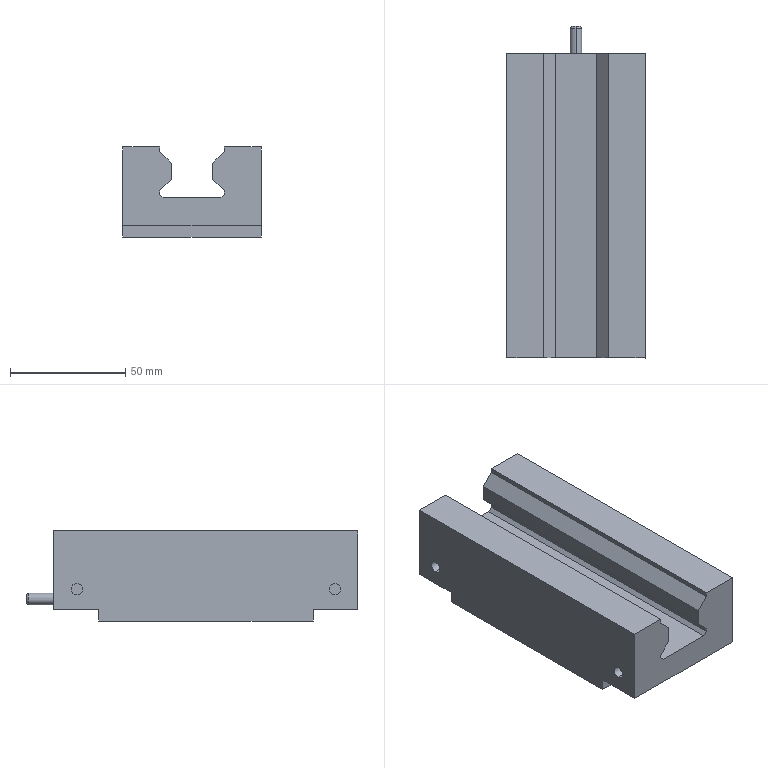Part | SolidWorks | features BaseBody 1 | 1 solid | 83 faces | box 60 x 143.8 x 39 mm | volume 227326 mm3 | plane 31 | cone 26 | cylinder 26 | commonest cylinder face diameters 6.8 x12 5 x10 10 x4